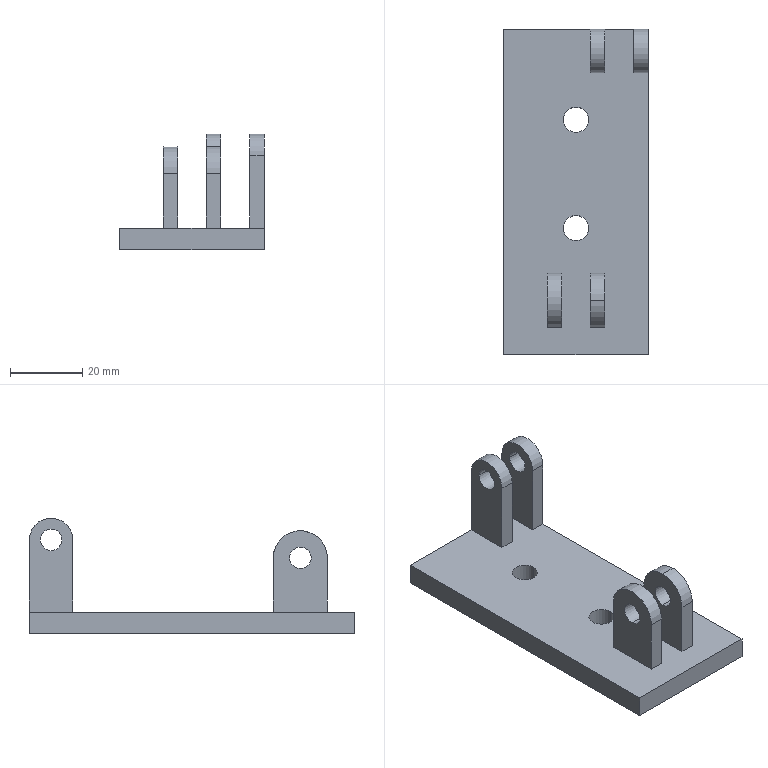Part | SolidWorks | features ICE 3, Extrusion 1, LPattern 1, MirrorPattern 1 | 1 solid | 36 faces | box 40 x 90 x 32 mm | volume 25565 mm3 | plane 19 | cylinder 17 | commonest cylinder face diameters 6 x8 7 x4 15 x3 12 x2
STEP:
#1=CARTESIAN_POINT('',(-3.5,20.,0.));
#2=VERTEX_POINT('',#1);
#3=CARTESIAN_POINT('',(3.5,20.,0.));
#4=VERTEX_POINT('',#3);
#5=CARTESIAN_POINT('',(0.,20.,0.));
#6=DIRECTION('',(0.,0.,1.));
#7=DIRECTION('',(1.,0.,0.));
#8=AXIS2_PLACEMENT_3D('',#5,#6,#7);
#9=CIRCLE('',#8,3.5);
#10=EDGE_CURVE('',#2,#4,#9,.T.);
#11=ORIENTED_EDGE('',*,*,#10,.F.);
#12=CARTESIAN_POINT('',(-3.5,20.,6.));
#13=VERTEX_POINT('',#12);
#14=CARTESIAN_POINT('',(-3.5,20.,0.));
#15=DIRECTION('',(0.,0.,1.));
#16=VECTOR('',#15,1000.);
#17=LINE('',#14,#16);
#18=EDGE_CURVE('',#2,#13,#17,.T.);
#19=ORIENTED_EDGE('',*,*,#18,.T.);
#20=CARTESIAN_POINT('',(3.5,20.,6.));
#21=VERTEX_POINT('',#20);
#22=CARTESIAN_POINT('',(0.,20.,6.));
#23=DIRECTION('',(0.,0.,1.));
#24=DIRECTION('',(1.,0.,0.));
#25=AXIS2_PLACEMENT_3D('',#22,#23,#24);
#26=CIRCLE('',#25,3.5);
#27=EDGE_CURVE('',#13,#21,#26,.T.);
#28=ORIENTED_EDGE('',*,*,#27,.T.);
#29=CARTESIAN_POINT('',(3.5,20.,0.));
#30=DIRECTION('',(0.,0.,1.));
#31=VECTOR('',#30,1000.);
#32=LINE('',#29,#31);
#33=EDGE_CURVE('',#4,#21,#32,.T.);
#34=ORIENTED_EDGE('',*,*,#33,.F.);
#35=EDGE_LOOP('',(#11,#19,#28,#34));
#36=FACE_OUTER_BOUND('',#35,.T.);
#37=CARTESIAN_POINT('',(0.,20.,0.));
#38=DIRECTION('',(0.,0.,1.));
#39=DIRECTION('',(1.,0.,0.));
#40=AXIS2_PLACEMENT_3D('',#37,#38,#39);
#41=CYLINDRICAL_SURFACE('',#40,3.5);
#42=ADVANCED_FACE('',(#36),#41,.F.);
#43=CARTESIAN_POINT('',(-3.5,-10.,0.));
#44=VERTEX_POINT('',#43);
#45=CARTESIAN_POINT('',(3.5,-10.,0.));
#46=VERTEX_POINT('',#45);
#47=CARTESIAN_POINT('',(0.,-10.,0.));
#48=DIRECTION('',(0.,0.,1.));
#49=DIRECTION('',(1.,0.,0.));
#50=AXIS2_PLACEMENT_3D('',#47,#48,#49);
#51=CIRCLE('',#50,3.5);
#52=EDGE_CURVE('',#44,#46,#51,.T.);
#53=ORIENTED_EDGE('',*,*,#52,.F.);
#54=CARTESIAN_POINT('',(-3.5,-10.,6.));
#55=VERTEX_POINT('',#54);
#56=CARTESIAN_POINT('',(-3.5,-10.,0.));
#57=DIRECTION('',(0.,0.,1.));
#58=VECTOR('',#57,1000.);
#59=LINE('',#56,#58);
#60=EDGE_CURVE('',#44,#55,#59,.T.);
#61=ORIENTED_EDGE('',*,*,#60,.T.);
#62=CARTESIAN_POINT('',(3.5,-10.,6.));
#63=VERTEX_POINT('',#62);
#64=CARTESIAN_POINT('',(0.,-10.,6.));
#65=DIRECTION('',(0.,0.,1.));
#66=DIRECTION('',(1.,0.,0.));
#67=AXIS2_PLACEMENT_3D('',#64,#65,#66);
#68=CIRCLE('',#67,3.5);
#69=EDGE_CURVE('',#55,#63,#68,.T.);
#70=ORIENTED_EDGE('',*,*,#69,.T.);
#71=CARTESIAN_POINT('',(3.5,-10.,0.));
#72=DIRECTION('',(0.,0.,1.));
#73=VECTOR('',#72,1000.);
#74=LINE('',#71,#73);
#75=EDGE_CURVE('',#46,#63,#74,.T.);
#76=ORIENTED_EDGE('',*,*,#75,.F.);
#77=EDGE_LOOP('',(#53,#61,#70,#76));
#78=FACE_OUTER_BOUND('',#77,.T.);
#79=CARTESIAN_POINT('',(0.,-10.,0.));
#80=DIRECTION('',(0.,0.,1.));
#81=DIRECTION('',(1.,0.,0.));
#82=AXIS2_PLACEMENT_3D('',#79,#80,#81);
#83=CYLINDRICAL_SURFACE('',#82,3.5);
#84=ADVANCED_FACE('',(#78),#83,.F.);
#85=CARTESIAN_POINT('',(4.,42.,26.));
#86=VERTEX_POINT('',#85);
#87=CARTESIAN_POINT('',(4.,36.,26.));
#88=VERTEX_POINT('',#87);
#89=CARTESIAN_POINT('',(4.,39.,26.));
#90=DIRECTION('',(-1.,0.,0.));
#91=DIRECTION('',(0.,-1.,0.));
#92=AXIS2_PLACEMENT_3D('',#89,#90,#91);
#93=CIRCLE('',#92,3.);
#94=EDGE_CURVE('',#86,#88,#93,.T.);
#95=ORIENTED_EDGE('',*,*,#94,.T.);
#96=CARTESIAN_POINT('',(8.,36.,26.));
#97=VERTEX_POINT('',#96);
#98=CARTESIAN_POINT('',(4.,36.,26.));
#99=DIRECTION('',(1.,0.,0.));
#100=VECTOR('',#99,1000.);
#101=LINE('',#98,#100);
#102=EDGE_CURVE('',#88,#97,#101,.T.);
#103=ORIENTED_EDGE('',*,*,#102,.T.);
#104=CARTESIAN_POINT('',(8.,42.,26.));
#105=VERTEX_POINT('',#104);
#106=CARTESIAN_POINT('',(8.,39.,26.));
#107=DIRECTION('',(-1.,0.,0.));
#108=DIRECTION('',(0.,-1.,0.));
#109=AXIS2_PLACEMENT_3D('',#106,#107,#108);
#110=CIRCLE('',#109,3.);
#111=EDGE_CURVE('',#105,#97,#110,.T.);
#112=ORIENTED_EDGE('',*,*,#111,.F.);
#113=CARTESIAN_POINT('',(4.,42.,26.));
#114=DIRECTION('',(1.,0.,0.));
#115=VECTOR('',#114,1000.);
#116=LINE('',#113,#115);
#117=EDGE_CURVE('',#86,#105,#116,.T.);
#118=ORIENTED_EDGE('',*,*,#117,.F.);
#119=EDGE_LOOP('',(#95,#103,#112,#118));
#120=FACE_OUTER_BOUND('',#119,.T.);
#121=CARTESIAN_POINT('',(4.,39.,26.));
#122=DIRECTION('',(1.,0.,0.));
#123=DIRECTION('',(0.,1.,0.));
#124=AXIS2_PLACEMENT_3D('',#121,#122,#123);
#125=CYLINDRICAL_SURFACE('',#124,3.);
#126=ADVANCED_FACE('',(#120),#125,.F.);
#127=CARTESIAN_POINT('',(-8.,-30.,24.));
#128=VERTEX_POINT('',#127);
#129=CARTESIAN_POINT('',(-8.,-30.,18.));
#130=VERTEX_POINT('',#129);
#131=CARTESIAN_POINT('',(-8.,-30.,21.));
#132=DIRECTION('',(1.,0.,0.));
#133=DIRECTION('',(0.,0.,-1.));
#134=AXIS2_PLACEMENT_3D('',#131,#132,#133);
#135=CIRCLE('',#134,3.);
#136=EDGE_CURVE('',#128,#130,#135,.T.);
#137=ORIENTED_EDGE('',*,*,#136,.F.);
#138=CARTESIAN_POINT('',(-4.,-30.,24.));
#139=VERTEX_POINT('',#138);
#140=CARTESIAN_POINT('',(-8.,-30.,24.));
#141=DIRECTION('',(1.,0.,0.));
#142=VECTOR('',#141,1000.);
#143=LINE('',#140,#142);
#144=EDGE_CURVE('',#128,#139,#143,.T.);
#145=ORIENTED_EDGE('',*,*,#144,.T.);
#146=CARTESIAN_POINT('',(-4.,-30.,18.));
#147=VERTEX_POINT('',#146);
#148=CARTESIAN_POINT('',(-4.,-30.,21.));
#149=DIRECTION('',(1.,0.,0.));
#150=DIRECTION('',(0.,0.,-1.));
#151=AXIS2_PLACEMENT_3D('',#148,#149,#150);
#152=CIRCLE('',#151,3.);
#153=EDGE_CURVE('',#139,#147,#152,.T.);
#154=ORIENTED_EDGE('',*,*,#153,.T.);
#155=CARTESIAN_POINT('',(-8.,-30.,18.));
#156=DIRECTION('',(1.,0.,0.));
#157=VECTOR('',#156,1000.);
#158=LINE('',#155,#157);
#159=EDGE_CURVE('',#130,#147,#158,.T.);
#160=ORIENTED_EDGE('',*,*,#159,.F.);
#161=EDGE_LOOP('',(#137,#145,#154,#160));
#162=FACE_OUTER_BOUND('',#161,.T.);
#163=CARTESIAN_POINT('',(-8.,-30.,21.));
#164=DIRECTION('',(1.,0.,0.));
#165=DIRECTION('',(0.,0.,-1.));
#166=AXIS2_PLACEMENT_3D('',#163,#164,#165);
#167=CYLINDRICAL_SURFACE('',#166,3.);
#168=ADVANCED_FACE('',(#162),#167,.F.);
#169=CARTESIAN_POINT('',(8.,-30.,24.));
#170=VERTEX_POINT('',#169);
#171=CARTESIAN_POINT('',(8.,-30.,18.));
#172=VERTEX_POINT('',#171);
#173=CARTESIAN_POINT('',(8.,-30.,21.));
#174=DIRECTION('',(1.,0.,0.));
#175=DIRECTION('',(0.,0.,-1.));
#176=AXIS2_PLACEMENT_3D('',#173,#174,#175);
#177=CIRCLE('',#176,3.);
#178=EDGE_CURVE('',#170,#172,#177,.T.);
#179=ORIENTED_EDGE('',*,*,#178,.T.);
#180=CARTESIAN_POINT('',(4.,-30.,18.));
#181=VERTEX_POINT('',#180);
#182=CARTESIAN_POINT('',(8.,-30.,18.));
#183=DIRECTION('',(-1.,0.,0.));
#184=VECTOR('',#183,1000.);
#185=LINE('',#182,#184);
#186=EDGE_CURVE('',#172,#181,#185,.T.);
#187=ORIENTED_EDGE('',*,*,#186,.T.);
#188=CARTESIAN_POINT('',(4.,-30.,24.));
#189=VERTEX_POINT('',#188);
#190=CARTESIAN_POINT('',(4.,-30.,21.));
#191=DIRECTION('',(1.,0.,0.));
#192=DIRECTION('',(0.,0.,-1.));
#193=AXIS2_PLACEMENT_3D('',#190,#191,#192);
#194=CIRCLE('',#193,3.);
#195=EDGE_CURVE('',#189,#181,#194,.T.);
#196=ORIENTED_EDGE('',*,*,#195,.F.);
#197=CARTESIAN_POINT('',(8.,-30.,24.));
#198=DIRECTION('',(-1.,0.,0.));
#199=VECTOR('',#198,1000.);
#200=LINE('',#197,#199);
#201=EDGE_CURVE('',#170,#189,#200,.T.);
#202=ORIENTED_EDGE('',*,*,#201,.F.);
#203=EDGE_LOOP('',(#179,#187,#196,#202));
#204=FACE_OUTER_BOUND('',#203,.T.);
#205=CARTESIAN_POINT('',(8.,-30.,21.));
#206=DIRECTION('',(-1.,0.,0.));
#207=DIRECTION('',(0.,0.,1.));
#208=AXIS2_PLACEMENT_3D('',#205,#206,#207);
#209=CYLINDRICAL_SURFACE('',#208,3.);
#210=ADVANCED_FACE('',(#204),#209,.F.);
#211=CARTESIAN_POINT('',(8.,-30.,28.5));
#212=VERTEX_POINT('',#211);
#213=CARTESIAN_POINT('',(8.,-37.5,21.));
#214=VERTEX_POINT('',#213);
#215=CARTESIAN_POINT('',(8.,-30.,21.));
#216=DIRECTION('',(1.,0.,0.));
#217=DIRECTION('',(0.,0.,-1.));
#218=AXIS2_PLACEMENT_3D('',#215,#216,#217);
#219=CIRCLE('',#218,7.5);
#220=EDGE_CURVE('',#212,#214,#219,.T.);
#221=ORIENTED_EDGE('',*,*,#220,.F.);
#222=CARTESIAN_POINT('',(4.,-30.,28.5));
#223=VERTEX_POINT('',#222);
#224=CARTESIAN_POINT('',(8.,-30.,28.5));
#225=DIRECTION('',(-1.,0.,0.));
#226=VECTOR('',#225,1000.);
#227=LINE('',#224,#226);
#228=EDGE_CURVE('',#212,#223,#227,.T.);
#229=ORIENTED_EDGE('',*,*,#228,.T.);
#230=CARTESIAN_POINT('',(4.,-37.5,21.));
#231=VERTEX_POINT('',#230);
#232=CARTESIAN_POINT('',(4.,-30.,21.));
#233=DIRECTION('',(1.,0.,0.));
#234=DIRECTION('',(0.,0.,-1.));
#235=AXIS2_PLACEMENT_3D('',#232,#233,#234);
#236=CIRCLE('',#235,7.5);
#237=EDGE_CURVE('',#223,#231,#236,.T.);
#238=ORIENTED_EDGE('',*,*,#237,.T.);
#239=CARTESIAN_POINT('',(8.,-37.5,21.));
#240=DIRECTION('',(-1.,0.,0.));
#241=VECTOR('',#240,1000.);
#242=LINE('',#239,#241);
#243=EDGE_CURVE('',#214,#231,#242,.T.);
#244=ORIENTED_EDGE('',*,*,#243,.F.);
#245=EDGE_LOOP('',(#221,#229,#238,#244));
#246=FACE_OUTER_BOUND('',#245,.T.);
#247=CARTESIAN_POINT('',(8.,-30.,21.));
#248=DIRECTION('',(-1.,0.,0.));
#249=DIRECTION('',(0.,0.,1.));
#250=AXIS2_PLACEMENT_3D('',#247,#248,#249);
#251=CYLINDRICAL_SURFACE('',#250,7.5);
#252=ADVANCED_FACE('',(#246),#251,.T.);
#253=CARTESIAN_POINT('',(16.,42.,26.));
#254=VERTEX_POINT('',#253);
#255=CARTESIAN_POINT('',(16.,36.,26.));
#256=VERTEX_POINT('',#255);
#257=CARTESIAN_POINT('',(16.,39.,26.));
#258=DIRECTION('',(-1.,0.,0.));
#259=DIRECTION('',(0.,-1.,0.));
#260=AXIS2_PLACEMENT_3D('',#257,#258,#259);
#261=CIRCLE('',#260,3.);
#262=EDGE_CURVE('',#254,#256,#261,.T.);
#263=ORIENTED_EDGE('',*,*,#262,.T.);
#264=CARTESIAN_POINT('',(20.,36.,26.));
#265=VERTEX_POINT('',#264);
#266=CARTESIAN_POINT('',(16.,36.,26.));
#267=DIRECTION('',(1.,0.,0.));
#268=VECTOR('',#267,1000.);
#269=LINE('',#266,#268);
#270=EDGE_CURVE('',#256,#265,#269,.T.);
#271=ORIENTED_EDGE('',*,*,#270,.T.);
#272=CARTESIAN_POINT('',(20.,42.,26.));
#273=VERTEX_POINT('',#272);
#274=CARTESIAN_POINT('',(20.,39.,26.));
#275=DIRECTION('',(-1.,0.,0.));
#276=DIRECTION('',(0.,-1.,0.));
#277=AXIS2_PLACEMENT_3D('',#274,#275,#276);
#278=CIRCLE('',#277,3.);
#279=EDGE_CURVE('',#273,#265,#278,.T.);
#280=ORIENTED_EDGE('',*,*,#279,.F.);
#281=CARTESIAN_POINT('',(16.,42.,26.));
#282=DIRECTION('',(1.,0.,0.));
#283=VECTOR('',#282,1000.);
#284=LINE('',#281,#283);
#285=EDGE_CURVE('',#254,#273,#284,.T.);
#286=ORIENTED_EDGE('',*,*,#285,.F.);
#287=EDGE_LOOP('',(#263,#271,#280,#286));
#288=FACE_OUTER_BOUND('',#287,.T.);
#289=CARTESIAN_POINT('',(16.,39.,26.));
#290=DIRECTION('',(1.,0.,0.));
#291=DIRECTION('',(0.,1.,0.));
#292=AXIS2_PLACEMENT_3D('',#289,#290,#291);
#293=CYLINDRICAL_SURFACE('',#292,3.);
#294=ADVANCED_FACE('',(#288),#293,.F.);
#295=CARTESIAN_POINT('',(0.,20.,6.));
#296=DIRECTION('',(0.,0.,1.));
#297=DIRECTION('',(1.,0.,0.));
#298=AXIS2_PLACEMENT_3D('',#295,#296,#297);
#299=CIRCLE('',#298,3.5);
#300=EDGE_CURVE('',#21,#13,#299,.T.);
#301=ORIENTED_EDGE('',*,*,#300,.F.);
#302=ORIENTED_EDGE('',*,*,#27,.F.);
#303=EDGE_LOOP('',(#301,#302));
#304=FACE_BOUND('',#303,.T.);
#305=CARTESIAN_POINT('',(0.,-10.,6.));
#306=DIRECTION('',(0.,0.,1.));
#307=DIRECTION('',(1.,0.,0.));
#308=AXIS2_PLACEMENT_3D('',#305,#306,#307);
#309=CIRCLE('',#308,3.5);
#310=EDGE_CURVE('',#63,#55,#309,.T.);
#311=ORIENTED_EDGE('',*,*,#310,.F.);
#312=ORIENTED_EDGE('',*,*,#69,.F.);
#313=EDGE_LOOP('',(#311,#312));
#314=FACE_BOUND('',#313,.T.);
#315=CARTESIAN_POINT('',(4.,45.,6.));
#316=VERTEX_POINT('',#315);
#317=CARTESIAN_POINT('',(4.,33.,6.));
#318=VERTEX_POINT('',#317);
#319=CARTESIAN_POINT('',(4.,45.,6.));
#320=DIRECTION('',(0.,-1.,0.));
#321=VECTOR('',#320,1000.);
#322=LINE('',#319,#321);
#323=EDGE_CURVE('',#316,#318,#322,.T.);
#324=ORIENTED_EDGE('',*,*,#323,.F.);
#325=CARTESIAN_POINT('',(-20.,45.,6.));
#326=VERTEX_POINT('',#325);
#327=CARTESIAN_POINT('',(-20.,45.,6.));
#328=DIRECTION('',(-1.,0.,0.));
#329=VECTOR('',#328,1000.);
#330=LINE('',#327,#329);
#331=EDGE_CURVE('',#316,#326,#330,.T.);
#332=ORIENTED_EDGE('',*,*,#331,.T.);
#333=CARTESIAN_POINT('',(-20.,-45.,6.));
#334=VERTEX_POINT('',#333);
#335=CARTESIAN_POINT('',(-20.,45.,6.));
#336=DIRECTION('',(0.,-1.,0.));
#337=VECTOR('',#336,1000.);
#338=LINE('',#335,#337);
#339=EDGE_CURVE('',#326,#334,#338,.T.);
#340=ORIENTED_EDGE('',*,*,#339,.T.);
#341=CARTESIAN_POINT('',(20.,-45.,6.));
#342=VERTEX_POINT('',#341);
#343=CARTESIAN_POINT('',(-20.,-45.,6.));
#344=DIRECTION('',(1.,0.,0.));
#345=VECTOR('',#344,1000.);
#346=LINE('',#343,#345);
#347=EDGE_CURVE('',#334,#342,#346,.T.);
#348=ORIENTED_EDGE('',*,*,#347,.T.);
#349=CARTESIAN_POINT('',(20.,33.,6.));
#350=VERTEX_POINT('',#349);
#351=CARTESIAN_POINT('',(20.,45.,6.));
#352=DIRECTION('',(0.,1.,0.));
#353=VECTOR('',#352,1000.);
#354=LINE('',#351,#353);
#355=EDGE_CURVE('',#342,#350,#354,.T.);
#356=ORIENTED_EDGE('',*,*,#355,.T.);
#357=CARTESIAN_POINT('',(16.,33.,6.));
#358=VERTEX_POINT('',#357);
#359=CARTESIAN_POINT('',(16.,33.,6.));
#360=DIRECTION('',(1.,0.,0.));
#361=VECTOR('',#360,1000.);
#362=LINE('',#359,#361);
#363=EDGE_CURVE('',#358,#350,#362,.T.);
#364=ORIENTED_EDGE('',*,*,#363,.F.);
#365=CARTESIAN_POINT('',(16.,45.,6.));
#366=VERTEX_POINT('',#365);
#367=CARTESIAN_POINT('',(16.,45.,6.));
#368=DIRECTION('',(0.,-1.,0.));
#369=VECTOR('',#368,1000.);
#370=LINE('',#367,#369);
#371=EDGE_CURVE('',#366,#358,#370,.T.);
#372=ORIENTED_EDGE('',*,*,#371,.F.);
#373=CARTESIAN_POINT('',(8.,45.,6.));
#374=VERTEX_POINT('',#373);
#375=CARTESIAN_POINT('',(-20.,45.,6.));
#376=DIRECTION('',(-1.,0.,0.));
#377=VECTOR('',#376,1000.);
#378=LINE('',#375,#377);
#379=EDGE_CURVE('',#366,#374,#378,.T.);
#380=ORIENTED_EDGE('',*,*,#379,.T.);
#381=CARTESIAN_POINT('',(8.,33.,6.));
#382=VERTEX_POINT('',#381);
#383=CARTESIAN_POINT('',(8.,45.,6.));
#384=DIRECTION('',(0.,-1.,0.));
#385=VECTOR('',#384,1000.);
#386=LINE('',#383,#385);
#387=EDGE_CURVE('',#374,#382,#386,.T.);
#388=ORIENTED_EDGE('',*,*,#387,.T.);
#389=CARTESIAN_POINT('',(4.,33.,6.));
#390=DIRECTION('',(1.,0.,0.));
#391=VECTOR('',#390,1000.);
#392=LINE('',#389,#391);
#393=EDGE_CURVE('',#318,#382,#392,.T.);
#394=ORIENTED_EDGE('',*,*,#393,.F.);
#395=EDGE_LOOP('',(#324,#332,#340,#348,#356,#364,#372,#380,#388,#394));
#396=FACE_OUTER_BOUND('',#395,.T.);
#397=CARTESIAN_POINT('',(-8.,-37.5,6.));
#398=VERTEX_POINT('',#397);
#399=CARTESIAN_POINT('',(-8.,-22.5,6.));
#400=VERTEX_POINT('',#399);
#401=CARTESIAN_POINT('',(-8.,-22.5,6.));
#402=DIRECTION('',(0.,1.,0.));
#403=VECTOR('',#402,1000.);
#404=LINE('',#401,#403);
#405=EDGE_CURVE('',#398,#400,#404,.T.);
#406=ORIENTED_EDGE('',*,*,#405,.T.);
#407=CARTESIAN_POINT('',(-4.,-22.5,6.));
#408=VERTEX_POINT('',#407);
#409=CARTESIAN_POINT('',(-8.,-22.5,6.));
#410=DIRECTION('',(1.,0.,0.));
#411=VECTOR('',#410,1000.);
#412=LINE('',#409,#411);
#413=EDGE_CURVE('',#400,#408,#412,.T.);
#414=ORIENTED_EDGE('',*,*,#413,.T.);
#415=CARTESIAN_POINT('',(-4.,-37.5,6.));
#416=VERTEX_POINT('',#415);
#417=CARTESIAN_POINT('',(-4.,-22.5,6.));
#418=DIRECTION('',(0.,1.,0.));
#419=VECTOR('',#418,1000.);
#420=LINE('',#417,#419);
#421=EDGE_CURVE('',#416,#408,#420,.T.);
#422=ORIENTED_EDGE('',*,*,#421,.F.);
#423=CARTESIAN_POINT('',(-8.,-37.5,6.));
#424=DIRECTION('',(1.,0.,0.));
#425=VECTOR('',#424,1000.);
#426=LINE('',#423,#425);
#427=EDGE_CURVE('',#398,#416,#426,.T.);
#428=ORIENTED_EDGE('',*,*,#427,.F.);
#429=EDGE_LOOP('',(#406,#414,#422,#428));
#430=FACE_BOUND('',#429,.T.);
#431=CARTESIAN_POINT('',(8.,-37.5,6.));
#432=VERTEX_POINT('',#431);
#433=CARTESIAN_POINT('',(8.,-22.5,6.));
#434=VERTEX_POINT('',#433);
#435=CARTESIAN_POINT('',(8.,-22.5,6.));
#436=DIRECTION('',(0.,1.,0.));
#437=VECTOR('',#436,1000.);
#438=LINE('',#435,#437);
#439=EDGE_CURVE('',#432,#434,#438,.T.);
#440=ORIENTED_EDGE('',*,*,#439,.F.);
#441=CARTESIAN_POINT('',(4.,-37.5,6.));
#442=VERTEX_POINT('',#441);
#443=CARTESIAN_POINT('',(8.,-37.5,6.));
#444=DIRECTION('',(-1.,0.,0.));
#445=VECTOR('',#444,1000.);
#446=LINE('',#443,#445);
#447=EDGE_CURVE('',#432,#442,#446,.T.);
#448=ORIENTED_EDGE('',*,*,#447,.T.);
#449=CARTESIAN_POINT('',(4.,-22.5,6.));
#450=VERTEX_POINT('',#449);
#451=CARTESIAN_POINT('',(4.,-22.5,6.));
#452=DIRECTION('',(0.,1.,0.));
#453=VECTOR('',#452,1000.);
#454=LINE('',#451,#453);
#455=EDGE_CURVE('',#442,#450,#454,.T.);
#456=ORIENTED_EDGE('',*,*,#455,.T.);
#457=CARTESIAN_POINT('',(8.,-22.5,6.));
#458=DIRECTION('',(-1.,0.,0.));
#459=VECTOR('',#458,1000.);
#460=LINE('',#457,#459);
#461=EDGE_CURVE('',#434,#450,#460,.T.);
#462=ORIENTED_EDGE('',*,*,#461,.F.);
#463=EDGE_LOOP('',(#440,#448,#456,#462));
#464=FACE_BOUND('',#463,.T.);
#465=CARTESIAN_POINT('',(0.,0.,6.));
#466=DIRECTION('',(0.,0.,1.));
#467=DIRECTION('',(1.,0.,0.));
#468=AXIS2_PLACEMENT_3D('',#465,#466,#467);
#469=PLANE('',#468);
#470=ADVANCED_FACE('',(#304,#314,#396,#430,#464),#469,.T.);
#471=CARTESIAN_POINT('',(20.,-45.,0.));
#472=VERTEX_POINT('',#471);
#473=CARTESIAN_POINT('',(20.,45.,0.));
#474=VERTEX_POINT('',#473);
#475=CARTESIAN_POINT('',(20.,45.,0.));
#476=DIRECTION('',(0.,1.,0.));
#477=VECTOR('',#476,1000.);
#478=LINE('',#475,#477);
#479=EDGE_CURVE('',#472,#474,#478,.T.);
#480=ORIENTED_EDGE('',*,*,#479,.T.);
#481=CARTESIAN_POINT('',(20.,45.,26.));
#482=VERTEX_POINT('',#481);
#483=CARTESIAN_POINT('',(20.,45.,6.));
#484=DIRECTION('',(0.,0.,-1.));
#485=VECTOR('',#484,1000.);
#486=LINE('',#483,#485);
#487=EDGE_CURVE('',#482,#474,#486,.T.);
#488=ORIENTED_EDGE('',*,*,#487,.F.);
#489=CARTESIAN_POINT('',(20.,33.,26.));
#490=VERTEX_POINT('',#489);
#491=CARTESIAN_POINT('',(20.,39.,26.));
#492=DIRECTION('',(-1.,0.,0.));
#493=DIRECTION('',(0.,-1.,0.));
#494=AXIS2_PLACEMENT_3D('',#491,#492,#493);
#495=CIRCLE('',#494,6.);
#496=EDGE_CURVE('',#490,#482,#495,.T.);
#497=ORIENTED_EDGE('',*,*,#496,.F.);
#498=CARTESIAN_POINT('',(20.,33.,6.));
#499=DIRECTION('',(0.,0.,1.));
#500=VECTOR('',#499,1000.);
#501=LINE('',#498,#500);
#502=EDGE_CURVE('',#350,#490,#501,.T.);
#503=ORIENTED_EDGE('',*,*,#502,.F.);
#504=ORIENTED_EDGE('',*,*,#355,.F.);
#505=CARTESIAN_POINT('',(20.,-45.,6.));
#506=DIRECTION('',(0.,0.,-1.));
#507=VECTOR('',#506,1000.);
#508=LINE('',#505,#507);
#509=EDGE_CURVE('',#342,#472,#508,.T.);
#510=ORIENTED_EDGE('',*,*,#509,.T.);
#511=EDGE_LOOP('',(#480,#488,#497,#503,#504,#510));
#512=FACE_OUTER_BOUND('',#511,.T.);
#513=ORIENTED_EDGE('',*,*,#279,.T.);
#514=CARTESIAN_POINT('',(20.,39.,26.));
#515=DIRECTION('',(-1.,0.,0.));
#516=DIRECTION('',(0.,-1.,0.));
#517=AXIS2_PLACEMENT_3D('',#514,#515,#516);
#518=CIRCLE('',#517,3.);
#519=EDGE_CURVE('',#265,#273,#518,.T.);
#520=ORIENTED_EDGE('',*,*,#519,.T.);
#521=EDGE_LOOP('',(#513,#520));
#522=FACE_BOUND('',#521,.T.);
#523=CARTESIAN_POINT('',(20.,45.,6.));
#524=DIRECTION('',(-1.,0.,0.));
#525=DIRECTION('',(0.,-1.,0.));
#526=AXIS2_PLACEMENT_3D('',#523,#524,#525);
#527=PLANE('',#526);
#528=ADVANCED_FACE('',(#512,#522),#527,.F.);
#529=CARTESIAN_POINT('',(-20.,45.,0.));
#530=VERTEX_POINT('',#529);
#531=CARTESIAN_POINT('',(-20.,45.,0.));
#532=DIRECTION('',(-1.,0.,0.));
#533=VECTOR('',#532,1000.);
#534=LINE('',#531,#533);
#535=EDGE_CURVE('',#474,#530,#534,.T.);
#536=ORIENTED_EDGE('',*,*,#535,.T.);
#537=CARTESIAN_POINT('',(-20.,45.,6.));
#538=DIRECTION('',(0.,0.,-1.));
#539=VECTOR('',#538,1000.);
#540=LINE('',#537,#539);
#541=EDGE_CURVE('',#326,#530,#540,.T.);
#542=ORIENTED_EDGE('',*,*,#541,.F.);
#543=ORIENTED_EDGE('',*,*,#331,.F.);
#544=CARTESIAN_POINT('',(4.,45.,26.));
#545=VERTEX_POINT('',#544);
#546=CARTESIAN_POINT('',(4.,45.,26.));
#547=DIRECTION('',(0.,0.,-1.));
#548=VECTOR('',#547,1000.);
#549=LINE('',#546,#548);
#550=EDGE_CURVE('',#545,#316,#549,.T.);
#551=ORIENTED_EDGE('',*,*,#550,.F.);
#552=CARTESIAN_POINT('',(8.,45.,26.));
#553=VERTEX_POINT('',#552);
#554=CARTESIAN_POINT('',(4.,45.,26.));
#555=DIRECTION('',(1.,0.,0.));
#556=VECTOR('',#555,1000.);
#557=LINE('',#554,#556);
#558=EDGE_CURVE('',#545,#553,#557,.T.);
#559=ORIENTED_EDGE('',*,*,#558,.T.);
#560=CARTESIAN_POINT('',(8.,45.,26.));
#561=DIRECTION('',(0.,0.,-1.));
#562=VECTOR('',#561,1000.);
#563=LINE('',#560,#562);
#564=EDGE_CURVE('',#553,#374,#563,.T.);
#565=ORIENTED_EDGE('',*,*,#564,.T.);
#566=ORIENTED_EDGE('',*,*,#379,.F.);
#567=CARTESIAN_POINT('',(16.,45.,26.));
#568=VERTEX_POINT('',#567);
#569=CARTESIAN_POINT('',(16.,45.,26.));
#570=DIRECTION('',(0.,0.,-1.));
#571=VECTOR('',#570,1000.);
#572=LINE('',#569,#571);
#573=EDGE_CURVE('',#568,#366,#572,.T.);
#574=ORIENTED_EDGE('',*,*,#573,.F.);
#575=CARTESIAN_POINT('',(16.,45.,26.));
#576=DIRECTION('',(1.,0.,0.));
#577=VECTOR('',#576,1000.);
#578=LINE('',#575,#577);
#579=EDGE_CURVE('',#568,#482,#578,.T.);
#580=ORIENTED_EDGE('',*,*,#579,.T.);
#581=ORIENTED_EDGE('',*,*,#487,.T.);
#582=EDGE_LOOP('',(#536,#542,#543,#551,#559,#565,#566,#574,#580,#581));
#583=FACE_OUTER_BOUND('',#582,.T.);
#584=CARTESIAN_POINT('',(-20.,45.,6.));
#585=DIRECTION('',(0.,-1.,0.));
#586=DIRECTION('',(0.,0.,-1.));
#587=AXIS2_PLACEMENT_3D('',#584,#585,#586);
#588=PLANE('',#587);
#589=ADVANCED_FACE('',(#583),#588,.F.);
#590=CARTESIAN_POINT('',(-20.,-45.,0.));
#591=VERTEX_POINT('',#590);
#592=CARTESIAN_POINT('',(-20.,45.,0.));
#593=DIRECTION('',(0.,-1.,0.));
#594=VECTOR('',#593,1000.);
#595=LINE('',#592,#594);
#596=EDGE_CURVE('',#530,#591,#595,.T.);
#597=ORIENTED_EDGE('',*,*,#596,.T.);
#598=CARTESIAN_POINT('',(-20.,-45.,6.));
#599=DIRECTION('',(0.,0.,-1.));
#600=VECTOR('',#599,1000.);
#601=LINE('',#598,#600);
#602=EDGE_CURVE('',#334,#591,#601,.T.);
#603=ORIENTED_EDGE('',*,*,#602,.F.);
#604=ORIENTED_EDGE('',*,*,#339,.F.);
#605=ORIENTED_EDGE('',*,*,#541,.T.);
#606=EDGE_LOOP('',(#597,#603,#604,#605));
#607=FACE_OUTER_BOUND('',#606,.T.);
#608=CARTESIAN_POINT('',(-20.,45.,6.));
#609=DIRECTION('',(1.,0.,0.));
#610=DIRECTION('',(0.,1.,0.));
#611=AXIS2_PLACEMENT_3D('',#608,#609,#610);
#612=PLANE('',#611);
#613=ADVANCED_FACE('',(#607),#612,.F.);
#614=CARTESIAN_POINT('',(-20.,-45.,0.));
#615=DIRECTION('',(1.,0.,0.));
#616=VECTOR('',#615,1000.);
#617=LINE('',#614,#616);
#618=EDGE_CURVE('',#591,#472,#617,.T.);
#619=ORIENTED_EDGE('',*,*,#618,.T.);
#620=ORIENTED_EDGE('',*,*,#509,.F.);
#621=ORIENTED_EDGE('',*,*,#347,.F.);
#622=ORIENTED_EDGE('',*,*,#602,.T.);
#623=EDGE_LOOP('',(#619,#620,#621,#622));
#624=FACE_OUTER_BOUND('',#623,.T.);
#625=CARTESIAN_POINT('',(-20.,-45.,6.));
#626=DIRECTION('',(0.,1.,0.));
#627=DIRECTION('',(0.,0.,1.));
#628=AXIS2_PLACEMENT_3D('',#625,#626,#627);
#629=PLANE('',#628);
#630=ADVANCED_FACE('',(#624),#629,.F.);
#631=CARTESIAN_POINT('',(0.,20.,0.));
#632=DIRECTION('',(0.,0.,1.));
#633=DIRECTION('',(1.,0.,0.));
#634=AXIS2_PLACEMENT_3D('',#631,#632,#633);
#635=CIRCLE('',#634,3.5);
#636=EDGE_CURVE('',#4,#2,#635,.T.);
#637=ORIENTED_EDGE('',*,*,#636,.T.);
#638=ORIENTED_EDGE('',*,*,#10,.T.);
#639=EDGE_LOOP('',(#637,#638));
#640=FACE_BOUND('',#639,.T.);
#641=CARTESIAN_POINT('',(0.,-10.,0.));
#642=DIRECTION('',(0.,0.,1.));
#643=DIRECTION('',(1.,0.,0.));
#644=AXIS2_PLACEMENT_3D('',#641,#642,#643);
#645=CIRCLE('',#644,3.5);
#646=EDGE_CURVE('',#46,#44,#645,.T.);
#647=ORIENTED_EDGE('',*,*,#646,.T.);
#648=ORIENTED_EDGE('',*,*,#52,.T.);
#649=EDGE_LOOP('',(#647,#648));
#650=FACE_BOUND('',#649,.T.);
#651=ORIENTED_EDGE('',*,*,#479,.F.);
#652=ORIENTED_EDGE('',*,*,#618,.F.);
#653=ORIENTED_EDGE('',*,*,#596,.F.);
#654=ORIENTED_EDGE('',*,*,#535,.F.);
#655=EDGE_LOOP('',(#651,#652,#653,#654));
#656=FACE_OUTER_BOUND('',#655,.T.);
#657=CARTESIAN_POINT('',(0.,0.,0.));
#658=DIRECTION('',(0.,0.,1.));
#659=DIRECTION('',(1.,0.,0.));
#660=AXIS2_PLACEMENT_3D('',#657,#658,#659);
#661=PLANE('',#660);
#662=ADVANCED_FACE('',(#640,#650,#656),#661,.F.);
#663=CARTESIAN_POINT('',(16.,33.,26.));
#664=VERTEX_POINT('',#663);
#665=CARTESIAN_POINT('',(16.,39.,26.));
#666=DIRECTION('',(-1.,0.,0.));
#667=DIRECTION('',(0.,-1.,0.));
#668=AXIS2_PLACEMENT_3D('',#665,#666,#667);
#669=CIRCLE('',#668,6.);
#670=EDGE_CURVE('',#664,#568,#669,.T.);
#671=ORIENTED_EDGE('',*,*,#670,.T.);
#672=ORIENTED_EDGE('',*,*,#573,.T.);
#673=ORIENTED_EDGE('',*,*,#371,.T.);
#674=CARTESIAN_POINT('',(16.,33.,6.));
#675=DIRECTION('',(0.,0.,1.));
#676=VECTOR('',#675,1000.);
#677=LINE('',#674,#676);
#678=EDGE_CURVE('',#358,#664,#677,.T.);
#679=ORIENTED_EDGE('',*,*,#678,.T.);
#680=EDGE_LOOP('',(#671,#672,#673,#679));
#681=FACE_OUTER_BOUND('',#680,.T.);
#682=ORIENTED_EDGE('',*,*,#262,.F.);
#683=CARTESIAN_POINT('',(16.,39.,26.));
#684=DIRECTION('',(-1.,0.,0.));
#685=DIRECTION('',(0.,-1.,0.));
#686=AXIS2_PLACEMENT_3D('',#683,#684,#685);
#687=CIRCLE('',#686,3.);
#688=EDGE_CURVE('',#256,#254,#687,.T.);
#689=ORIENTED_EDGE('',*,*,#688,.F.);
#690=EDGE_LOOP('',(#682,#689));
#691=FACE_BOUND('',#690,.T.);
#692=CARTESIAN_POINT('',(16.,39.,26.));
#693=DIRECTION('',(-1.,0.,0.));
#694=DIRECTION('',(0.,-1.,0.));
#695=AXIS2_PLACEMENT_3D('',#692,#693,#694);
#696=PLANE('',#695);
#697=ADVANCED_FACE('',(#681,#691),#696,.T.);
#698=ORIENTED_EDGE('',*,*,#496,.T.);
#699=ORIENTED_EDGE('',*,*,#579,.F.);
#700=ORIENTED_EDGE('',*,*,#670,.F.);
#701=CARTESIAN_POINT('',(16.,33.,26.));
#702=DIRECTION('',(1.,0.,0.));
#703=VECTOR('',#702,1000.);
#704=LINE('',#701,#703);
#705=EDGE_CURVE('',#664,#490,#704,.T.);
#706=ORIENTED_EDGE('',*,*,#705,.T.);
#707=EDGE_LOOP('',(#698,#699,#700,#706));
#708=FACE_OUTER_BOUND('',#707,.T.);
#709=CARTESIAN_POINT('',(16.,39.,26.));
#710=DIRECTION('',(1.,0.,0.));
#711=DIRECTION('',(0.,1.,0.));
#712=AXIS2_PLACEMENT_3D('',#709,#710,#711);
#713=CYLINDRICAL_SURFACE('',#712,6.);
#714=ADVANCED_FACE('',(#708),#713,.T.);
#715=ORIENTED_EDGE('',*,*,#502,.T.);
#716=ORIENTED_EDGE('',*,*,#705,.F.);
#717=ORIENTED_EDGE('',*,*,#678,.F.);
#718=ORIENTED_EDGE('',*,*,#363,.T.);
#719=EDGE_LOOP('',(#715,#716,#717,#718));
#720=FACE_OUTER_BOUND('',#719,.T.);
#721=CARTESIAN_POINT('',(16.,33.,6.));
#722=DIRECTION('',(0.,1.,0.));
#723=DIRECTION('',(-1.,0.,0.));
#724=AXIS2_PLACEMENT_3D('',#721,#722,#723);
#725=PLANE('',#724);
#726=ADVANCED_FACE('',(#720),#725,.F.);
#727=ORIENTED_EDGE('',*,*,#270,.F.);
#728=ORIENTED_EDGE('',*,*,#688,.T.);
#729=ORIENTED_EDGE('',*,*,#285,.T.);
#730=ORIENTED_EDGE('',*,*,#519,.F.);
#731=EDGE_LOOP('',(#727,#728,#729,#730));
#732=FACE_OUTER_BOUND('',#731,.T.);
#733=CARTESIAN_POINT('',(16.,39.,26.));
#734=DIRECTION('',(1.,0.,0.));
#735=DIRECTION('',(0.,1.,0.));
#736=AXIS2_PLACEMENT_3D('',#733,#734,#735);
#737=CYLINDRICAL_SURFACE('',#736,3.);
#738=ADVANCED_FACE('',(#732),#737,.F.);
#739=CARTESIAN_POINT('',(8.,-22.5,21.));
#740=VERTEX_POINT('',#739);
#741=CARTESIAN_POINT('',(8.,-30.,21.));
#742=DIRECTION('',(1.,0.,0.));
#743=DIRECTION('',(0.,0.,-1.));
#744=AXIS2_PLACEMENT_3D('',#741,#742,#743);
#745=CIRCLE('',#744,7.5);
#746=EDGE_CURVE('',#740,#212,#745,.T.);
#747=ORIENTED_EDGE('',*,*,#746,.T.);
#748=ORIENTED_EDGE('',*,*,#220,.T.);
#749=CARTESIAN_POINT('',(8.,-37.5,6.));
#750=DIRECTION('',(0.,0.,-1.));
#751=VECTOR('',#750,1000.);
#752=LINE('',#749,#751);
#753=EDGE_CURVE('',#214,#432,#752,.T.);
#754=ORIENTED_EDGE('',*,*,#753,.T.);
#755=ORIENTED_EDGE('',*,*,#439,.T.);
#756=CARTESIAN_POINT('',(8.,-22.5,21.));
#757=DIRECTION('',(0.,0.,1.));
#758=VECTOR('',#757,1000.);
#759=LINE('',#756,#758);
#760=EDGE_CURVE('',#434,#740,#759,.T.);
#761=ORIENTED_EDGE('',*,*,#760,.T.);
#762=EDGE_LOOP('',(#747,#748,#754,#755,#761));
#763=FACE_OUTER_BOUND('',#762,.T.);
#764=ORIENTED_EDGE('',*,*,#178,.F.);
#765=CARTESIAN_POINT('',(8.,-30.,21.));
#766=DIRECTION('',(1.,0.,0.));
#767=DIRECTION('',(0.,0.,-1.));
#768=AXIS2_PLACEMENT_3D('',#765,#766,#767);
#769=CIRCLE('',#768,3.);
#770=EDGE_CURVE('',#172,#170,#769,.T.);
#771=ORIENTED_EDGE('',*,*,#770,.F.);
#772=EDGE_LOOP('',(#764,#771));
#773=FACE_BOUND('',#772,.T.);
#774=CARTESIAN_POINT('',(8.,-30.,21.));
#775=DIRECTION('',(1.,0.,0.));
#776=DIRECTION('',(0.,0.,-1.));
#777=AXIS2_PLACEMENT_3D('',#774,#775,#776);
#778=PLANE('',#777);
#779=ADVANCED_FACE('',(#763,#773),#778,.T.);
#780=CARTESIAN_POINT('',(4.,-22.5,21.));
#781=VERTEX_POINT('',#780);
#782=CARTESIAN_POINT('',(4.,-30.,21.));
#783=DIRECTION('',(1.,0.,0.));
#784=DIRECTION('',(0.,0.,-1.));
#785=AXIS2_PLACEMENT_3D('',#782,#783,#784);
#786=CIRCLE('',#785,7.5);
#787=EDGE_CURVE('',#781,#223,#786,.T.);
#788=ORIENTED_EDGE('',*,*,#787,.F.);
#789=CARTESIAN_POINT('',(4.,-22.5,21.));
#790=DIRECTION('',(0.,0.,1.));
#791=VECTOR('',#790,1000.);
#792=LINE('',#789,#791);
#793=EDGE_CURVE('',#450,#781,#792,.T.);
#794=ORIENTED_EDGE('',*,*,#793,.F.);
#795=ORIENTED_EDGE('',*,*,#455,.F.);
#796=CARTESIAN_POINT('',(4.,-37.5,6.));
#797=DIRECTION('',(0.,0.,-1.));
#798=VECTOR('',#797,1000.);
#799=LINE('',#796,#798);
#800=EDGE_CURVE('',#231,#442,#799,.T.);
#801=ORIENTED_EDGE('',*,*,#800,.F.);
#802=ORIENTED_EDGE('',*,*,#237,.F.);
#803=EDGE_LOOP('',(#788,#794,#795,#801,#802));
#804=FACE_OUTER_BOUND('',#803,.T.);
#805=ORIENTED_EDGE('',*,*,#195,.T.);
#806=CARTESIAN_POINT('',(4.,-30.,21.));
#807=DIRECTION('',(1.,0.,0.));
#808=DIRECTION('',(0.,0.,-1.));
#809=AXIS2_PLACEMENT_3D('',#806,#807,#808);
#810=CIRCLE('',#809,3.);
#811=EDGE_CURVE('',#181,#189,#810,.T.);
#812=ORIENTED_EDGE('',*,*,#811,.T.);
#813=EDGE_LOOP('',(#805,#812));
#814=FACE_BOUND('',#813,.T.);
#815=CARTESIAN_POINT('',(4.,-30.,21.));
#816=DIRECTION('',(1.,0.,0.));
#817=DIRECTION('',(0.,0.,-1.));
#818=AXIS2_PLACEMENT_3D('',#815,#816,#817);
#819=PLANE('',#818);
#820=ADVANCED_FACE('',(#804,#814),#819,.F.);
#821=ORIENTED_EDGE('',*,*,#228,.F.);
#822=ORIENTED_EDGE('',*,*,#746,.F.);
#823=CARTESIAN_POINT('',(8.,-22.5,21.));
#824=DIRECTION('',(-1.,0.,0.));
#825=VECTOR('',#824,1000.);
#826=LINE('',#823,#825);
#827=EDGE_CURVE('',#740,#781,#826,.T.);
#828=ORIENTED_EDGE('',*,*,#827,.T.);
#829=ORIENTED_EDGE('',*,*,#787,.T.);
#830=EDGE_LOOP('',(#821,#822,#828,#829));
#831=FACE_OUTER_BOUND('',#830,.T.);
#832=CARTESIAN_POINT('',(8.,-30.,21.));
#833=DIRECTION('',(-1.,0.,0.));
#834=DIRECTION('',(0.,0.,1.));
#835=AXIS2_PLACEMENT_3D('',#832,#833,#834);
#836=CYLINDRICAL_SURFACE('',#835,7.5);
#837=ADVANCED_FACE('',(#831),#836,.T.);
#838=ORIENTED_EDGE('',*,*,#800,.T.);
#839=ORIENTED_EDGE('',*,*,#447,.F.);
#840=ORIENTED_EDGE('',*,*,#753,.F.);
#841=ORIENTED_EDGE('',*,*,#243,.T.);
#842=EDGE_LOOP('',(#838,#839,#840,#841));
#843=FACE_OUTER_BOUND('',#842,.T.);
#844=CARTESIAN_POINT('',(8.,-37.5,6.));
#845=DIRECTION('',(0.,1.,0.));
#846=DIRECTION('',(0.,0.,1.));
#847=AXIS2_PLACEMENT_3D('',#844,#845,#846);
#848=PLANE('',#847);
#849=ADVANCED_FACE('',(#843),#848,.F.);
#850=ORIENTED_EDGE('',*,*,#793,.T.);
#851=ORIENTED_EDGE('',*,*,#827,.F.);
#852=ORIENTED_EDGE('',*,*,#760,.F.);
#853=ORIENTED_EDGE('',*,*,#461,.T.);
#854=EDGE_LOOP('',(#850,#851,#852,#853));
#855=FACE_OUTER_BOUND('',#854,.T.);
#856=CARTESIAN_POINT('',(8.,-22.5,21.));
#857=DIRECTION('',(0.,-1.,0.));
#858=DIRECTION('',(0.,0.,-1.));
#859=AXIS2_PLACEMENT_3D('',#856,#857,#858);
#860=PLANE('',#859);
#861=ADVANCED_FACE('',(#855),#860,.F.);
#862=ORIENTED_EDGE('',*,*,#186,.F.);
#863=ORIENTED_EDGE('',*,*,#770,.T.);
#864=ORIENTED_EDGE('',*,*,#201,.T.);
#865=ORIENTED_EDGE('',*,*,#811,.F.);
#866=EDGE_LOOP('',(#862,#863,#864,#865));
#867=FACE_OUTER_BOUND('',#866,.T.);
#868=CARTESIAN_POINT('',(8.,-30.,21.));
#869=DIRECTION('',(-1.,0.,0.));
#870=DIRECTION('',(0.,0.,1.));
#871=AXIS2_PLACEMENT_3D('',#868,#869,#870);
#872=CYLINDRICAL_SURFACE('',#871,3.);
#873=ADVANCED_FACE('',(#867),#872,.F.);
#874=CARTESIAN_POINT('',(-4.,-22.5,21.));
#875=VERTEX_POINT('',#874);
#876=CARTESIAN_POINT('',(-4.,-37.5,21.));
#877=VERTEX_POINT('',#876);
#878=CARTESIAN_POINT('',(-4.,-30.,21.));
#879=DIRECTION('',(1.,0.,0.));
#880=DIRECTION('',(0.,0.,-1.));
#881=AXIS2_PLACEMENT_3D('',#878,#879,#880);
#882=CIRCLE('',#881,7.5);
#883=EDGE_CURVE('',#875,#877,#882,.T.);
#884=ORIENTED_EDGE('',*,*,#883,.F.);
#885=CARTESIAN_POINT('',(-8.,-22.5,21.));
#886=VERTEX_POINT('',#885);
#887=CARTESIAN_POINT('',(-8.,-22.5,21.));
#888=DIRECTION('',(1.,0.,0.));
#889=VECTOR('',#888,1000.);
#890=LINE('',#887,#889);
#891=EDGE_CURVE('',#886,#875,#890,.T.);
#892=ORIENTED_EDGE('',*,*,#891,.F.);
#893=CARTESIAN_POINT('',(-8.,-37.5,21.));
#894=VERTEX_POINT('',#893);
#895=CARTESIAN_POINT('',(-8.,-30.,21.));
#896=DIRECTION('',(1.,0.,0.));
#897=DIRECTION('',(0.,0.,-1.));
#898=AXIS2_PLACEMENT_3D('',#895,#896,#897);
#899=CIRCLE('',#898,7.5);
#900=EDGE_CURVE('',#886,#894,#899,.T.);
#901=ORIENTED_EDGE('',*,*,#900,.T.);
#902=CARTESIAN_POINT('',(-8.,-37.5,21.));
#903=DIRECTION('',(1.,0.,0.));
#904=VECTOR('',#903,1000.);
#905=LINE('',#902,#904);
#906=EDGE_CURVE('',#894,#877,#905,.T.);
#907=ORIENTED_EDGE('',*,*,#906,.T.);
#908=EDGE_LOOP('',(#884,#892,#901,#907));
#909=FACE_OUTER_BOUND('',#908,.T.);
#910=CARTESIAN_POINT('',(-8.,-30.,21.));
#911=DIRECTION('',(1.,0.,0.));
#912=DIRECTION('',(0.,0.,-1.));
#913=AXIS2_PLACEMENT_3D('',#910,#911,#912);
#914=CYLINDRICAL_SURFACE('',#913,7.5);
#915=ADVANCED_FACE('',(#909),#914,.T.);
#916=CARTESIAN_POINT('',(-4.,-22.5,21.));
#917=DIRECTION('',(0.,0.,1.));
#918=VECTOR('',#917,1000.);
#919=LINE('',#916,#918);
#920=EDGE_CURVE('',#408,#875,#919,.T.);
#921=ORIENTED_EDGE('',*,*,#920,.F.);
#922=ORIENTED_EDGE('',*,*,#413,.F.);
#923=CARTESIAN_POINT('',(-8.,-22.5,21.));
#924=DIRECTION('',(0.,0.,1.));
#925=VECTOR('',#924,1000.);
#926=LINE('',#923,#925);
#927=EDGE_CURVE('',#400,#886,#926,.T.);
#928=ORIENTED_EDGE('',*,*,#927,.T.);
#929=ORIENTED_EDGE('',*,*,#891,.T.);
#930=EDGE_LOOP('',(#921,#922,#928,#929));
#931=FACE_OUTER_BOUND('',#930,.T.);
#932=CARTESIAN_POINT('',(-8.,-22.5,21.));
#933=DIRECTION('',(0.,1.,0.));
#934=DIRECTION('',(0.,0.,1.));
#935=AXIS2_PLACEMENT_3D('',#932,#933,#934);
#936=PLANE('',#935);
#937=ADVANCED_FACE('',(#931),#936,.T.);
#938=CARTESIAN_POINT('',(-4.,-37.5,6.));
#939=DIRECTION('',(0.,0.,-1.));
#940=VECTOR('',#939,1000.);
#941=LINE('',#938,#940);
#942=EDGE_CURVE('',#877,#416,#941,.T.);
#943=ORIENTED_EDGE('',*,*,#942,.F.);
#944=ORIENTED_EDGE('',*,*,#906,.F.);
#945=CARTESIAN_POINT('',(-8.,-37.5,6.));
#946=DIRECTION('',(0.,0.,-1.));
#947=VECTOR('',#946,1000.);
#948=LINE('',#945,#947);
#949=EDGE_CURVE('',#894,#398,#948,.T.);
#950=ORIENTED_EDGE('',*,*,#949,.T.);
#951=ORIENTED_EDGE('',*,*,#427,.T.);
#952=EDGE_LOOP('',(#943,#944,#950,#951));
#953=FACE_OUTER_BOUND('',#952,.T.);
#954=CARTESIAN_POINT('',(-8.,-37.5,6.));
#955=DIRECTION('',(0.,-1.,0.));
#956=DIRECTION('',(0.,0.,-1.));
#957=AXIS2_PLACEMENT_3D('',#954,#955,#956);
#958=PLANE('',#957);
#959=ADVANCED_FACE('',(#953),#958,.T.);
#960=CARTESIAN_POINT('',(-8.,-30.,21.));
#961=DIRECTION('',(1.,0.,0.));
#962=DIRECTION('',(0.,0.,-1.));
#963=AXIS2_PLACEMENT_3D('',#960,#961,#962);
#964=CIRCLE('',#963,3.);
#965=EDGE_CURVE('',#130,#128,#964,.T.);
#966=ORIENTED_EDGE('',*,*,#965,.T.);
#967=ORIENTED_EDGE('',*,*,#136,.T.);
#968=EDGE_LOOP('',(#966,#967));
#969=FACE_BOUND('',#968,.T.);
#970=ORIENTED_EDGE('',*,*,#900,.F.);
#971=ORIENTED_EDGE('',*,*,#927,.F.);
#972=ORIENTED_EDGE('',*,*,#405,.F.);
#973=ORIENTED_EDGE('',*,*,#949,.F.);
#974=EDGE_LOOP('',(#970,#971,#972,#973));
#975=FACE_OUTER_BOUND('',#974,.T.);
#976=CARTESIAN_POINT('',(-8.,-30.,21.));
#977=DIRECTION('',(-1.,0.,0.));
#978=DIRECTION('',(0.,0.,-1.));
#979=AXIS2_PLACEMENT_3D('',#976,#977,#978);
#980=PLANE('',#979);
#981=ADVANCED_FACE('',(#969,#975),#980,.T.);
#982=CARTESIAN_POINT('',(-4.,-30.,21.));
#983=DIRECTION('',(1.,0.,0.));
#984=DIRECTION('',(0.,0.,-1.));
#985=AXIS2_PLACEMENT_3D('',#982,#983,#984);
#986=CIRCLE('',#985,3.);
#987=EDGE_CURVE('',#147,#139,#986,.T.);
#988=ORIENTED_EDGE('',*,*,#987,.F.);
#989=ORIENTED_EDGE('',*,*,#153,.F.);
#990=EDGE_LOOP('',(#988,#989));
#991=FACE_BOUND('',#990,.T.);
#992=ORIENTED_EDGE('',*,*,#883,.T.);
#993=ORIENTED_EDGE('',*,*,#942,.T.);
#994=ORIENTED_EDGE('',*,*,#421,.T.);
#995=ORIENTED_EDGE('',*,*,#920,.T.);
#996=EDGE_LOOP('',(#992,#993,#994,#995));
#997=FACE_OUTER_BOUND('',#996,.T.);
#998=CARTESIAN_POINT('',(-4.,-30.,21.));
#999=DIRECTION('',(-1.,0.,0.));
#1000=DIRECTION('',(0.,0.,-1.));
#1001=AXIS2_PLACEMENT_3D('',#998,#999,#1000);
#1002=PLANE('',#1001);
#1003=ADVANCED_FACE('',(#991,#997),#1002,.F.);
#1004=ORIENTED_EDGE('',*,*,#144,.F.);
#1005=ORIENTED_EDGE('',*,*,#965,.F.);
#1006=ORIENTED_EDGE('',*,*,#159,.T.);
#1007=ORIENTED_EDGE('',*,*,#987,.T.);
#1008=EDGE_LOOP('',(#1004,#1005,#1006,#1007));
#1009=FACE_OUTER_BOUND('',#1008,.T.);
#1010=CARTESIAN_POINT('',(-8.,-30.,21.));
#1011=DIRECTION('',(1.,0.,0.));
#1012=DIRECTION('',(0.,0.,-1.));
#1013=AXIS2_PLACEMENT_3D('',#1010,#1011,#1012);
#1014=CYLINDRICAL_SURFACE('',#1013,3.);
#1015=ADVANCED_FACE('',(#1009),#1014,.F.);
#1016=CARTESIAN_POINT('',(4.,33.,26.));
#1017=VERTEX_POINT('',#1016);
#1018=CARTESIAN_POINT('',(4.,39.,26.));
#1019=DIRECTION('',(-1.,0.,0.));
#1020=DIRECTION('',(0.,-1.,0.));
#1021=AXIS2_PLACEMENT_3D('',#1018,#1019,#1020);
#1022=CIRCLE('',#1021,6.);
#1023=EDGE_CURVE('',#1017,#545,#1022,.T.);
#1024=ORIENTED_EDGE('',*,*,#1023,.T.);
#1025=ORIENTED_EDGE('',*,*,#550,.T.);
#1026=ORIENTED_EDGE('',*,*,#323,.T.);
#1027=CARTESIAN_POINT('',(4.,33.,6.));
#1028=DIRECTION('',(0.,0.,1.));
#1029=VECTOR('',#1028,1000.);
#1030=LINE('',#1027,#1029);
#1031=EDGE_CURVE('',#318,#1017,#1030,.T.);
#1032=ORIENTED_EDGE('',*,*,#1031,.T.);
#1033=EDGE_LOOP('',(#1024,#1025,#1026,#1032));
#1034=FACE_OUTER_BOUND('',#1033,.T.);
#1035=ORIENTED_EDGE('',*,*,#94,.F.);
#1036=CARTESIAN_POINT('',(4.,39.,26.));
#1037=DIRECTION('',(-1.,0.,0.));
#1038=DIRECTION('',(0.,-1.,0.));
#1039=AXIS2_PLACEMENT_3D('',#1036,#1037,#1038);
#1040=CIRCLE('',#1039,3.);
#1041=EDGE_CURVE('',#88,#86,#1040,.T.);
#1042=ORIENTED_EDGE('',*,*,#1041,.F.);
#1043=EDGE_LOOP('',(#1035,#1042));
#1044=FACE_BOUND('',#1043,.T.);
#1045=CARTESIAN_POINT('',(4.,39.,26.));
#1046=DIRECTION('',(-1.,0.,0.));
#1047=DIRECTION('',(0.,-1.,0.));
#1048=AXIS2_PLACEMENT_3D('',#1045,#1046,#1047);
#1049=PLANE('',#1048);
#1050=ADVANCED_FACE('',(#1034,#1044),#1049,.T.);
#1051=CARTESIAN_POINT('',(8.,33.,26.));
#1052=VERTEX_POINT('',#1051);
#1053=CARTESIAN_POINT('',(8.,39.,26.));
#1054=DIRECTION('',(-1.,0.,0.));
#1055=DIRECTION('',(0.,-1.,0.));
#1056=AXIS2_PLACEMENT_3D('',#1053,#1054,#1055);
#1057=CIRCLE('',#1056,6.);
#1058=EDGE_CURVE('',#1052,#553,#1057,.T.);
#1059=ORIENTED_EDGE('',*,*,#1058,.F.);
#1060=CARTESIAN_POINT('',(8.,33.,6.));
#1061=DIRECTION('',(0.,0.,1.));
#1062=VECTOR('',#1061,1000.);
#1063=LINE('',#1060,#1062);
#1064=EDGE_CURVE('',#382,#1052,#1063,.T.);
#1065=ORIENTED_EDGE('',*,*,#1064,.F.);
#1066=ORIENTED_EDGE('',*,*,#387,.F.);
#1067=ORIENTED_EDGE('',*,*,#564,.F.);
#1068=EDGE_LOOP('',(#1059,#1065,#1066,#1067));
#1069=FACE_OUTER_BOUND('',#1068,.T.);
#1070=ORIENTED_EDGE('',*,*,#111,.T.);
#1071=CARTESIAN_POINT('',(8.,39.,26.));
#1072=DIRECTION('',(-1.,0.,0.));
#1073=DIRECTION('',(0.,-1.,0.));
#1074=AXIS2_PLACEMENT_3D('',#1071,#1072,#1073);
#1075=CIRCLE('',#1074,3.);
#1076=EDGE_CURVE('',#97,#105,#1075,.T.);
#1077=ORIENTED_EDGE('',*,*,#1076,.T.);
#1078=EDGE_LOOP('',(#1070,#1077));
#1079=FACE_BOUND('',#1078,.T.);
#1080=CARTESIAN_POINT('',(8.,39.,26.));
#1081=DIRECTION('',(-1.,0.,0.));
#1082=DIRECTION('',(0.,-1.,0.));
#1083=AXIS2_PLACEMENT_3D('',#1080,#1081,#1082);
#1084=PLANE('',#1083);
#1085=ADVANCED_FACE('',(#1069,#1079),#1084,.F.);
#1086=ORIENTED_EDGE('',*,*,#1058,.T.);
#1087=ORIENTED_EDGE('',*,*,#558,.F.);
#1088=ORIENTED_EDGE('',*,*,#1023,.F.);
#1089=CARTESIAN_POINT('',(4.,33.,26.));
#1090=DIRECTION('',(1.,0.,0.));
#1091=VECTOR('',#1090,1000.);
#1092=LINE('',#1089,#1091);
#1093=EDGE_CURVE('',#1017,#1052,#1092,.T.);
#1094=ORIENTED_EDGE('',*,*,#1093,.T.);
#1095=EDGE_LOOP('',(#1086,#1087,#1088,#1094));
#1096=FACE_OUTER_BOUND('',#1095,.T.);
#1097=CARTESIAN_POINT('',(4.,39.,26.));
#1098=DIRECTION('',(1.,0.,0.));
#1099=DIRECTION('',(0.,1.,0.));
#1100=AXIS2_PLACEMENT_3D('',#1097,#1098,#1099);
#1101=CYLINDRICAL_SURFACE('',#1100,6.);
#1102=ADVANCED_FACE('',(#1096),#1101,.T.);
#1103=ORIENTED_EDGE('',*,*,#1064,.T.);
#1104=ORIENTED_EDGE('',*,*,#1093,.F.);
#1105=ORIENTED_EDGE('',*,*,#1031,.F.);
#1106=ORIENTED_EDGE('',*,*,#393,.T.);
#1107=EDGE_LOOP('',(#1103,#1104,#1105,#1106));
#1108=FACE_OUTER_BOUND('',#1107,.T.);
#1109=CARTESIAN_POINT('',(4.,33.,6.));
#1110=DIRECTION('',(0.,1.,0.));
#1111=DIRECTION('',(-1.,0.,0.));
#1112=AXIS2_PLACEMENT_3D('',#1109,#1110,#1111);
#1113=PLANE('',#1112);
#1114=ADVANCED_FACE('',(#1108),#1113,.F.);
#1115=ORIENTED_EDGE('',*,*,#102,.F.);
#1116=ORIENTED_EDGE('',*,*,#1041,.T.);
#1117=ORIENTED_EDGE('',*,*,#117,.T.);
#1118=ORIENTED_EDGE('',*,*,#1076,.F.);
#1119=EDGE_LOOP('',(#1115,#1116,#1117,#1118));
#1120=FACE_OUTER_BOUND('',#1119,.T.);
#1121=CARTESIAN_POINT('',(4.,39.,26.));
#1122=DIRECTION('',(1.,0.,0.));
#1123=DIRECTION('',(0.,1.,0.));
#1124=AXIS2_PLACEMENT_3D('',#1121,#1122,#1123);
#1125=CYLINDRICAL_SURFACE('',#1124,3.);
#1126=ADVANCED_FACE('',(#1120),#1125,.F.);
#1127=ORIENTED_EDGE('',*,*,#60,.F.);
#1128=ORIENTED_EDGE('',*,*,#646,.F.);
#1129=ORIENTED_EDGE('',*,*,#75,.T.);
#1130=ORIENTED_EDGE('',*,*,#310,.T.);
#1131=EDGE_LOOP('',(#1127,#1128,#1129,#1130));
#1132=FACE_OUTER_BOUND('',#1131,.T.);
#1133=CARTESIAN_POINT('',(0.,-10.,0.));
#1134=DIRECTION('',(0.,0.,1.));
#1135=DIRECTION('',(1.,0.,0.));
#1136=AXIS2_PLACEMENT_3D('',#1133,#1134,#1135);
#1137=CYLINDRICAL_SURFACE('',#1136,3.5);
#1138=ADVANCED_FACE('',(#1132),#1137,.F.);
#1139=ORIENTED_EDGE('',*,*,#18,.F.);
#1140=ORIENTED_EDGE('',*,*,#636,.F.);
#1141=ORIENTED_EDGE('',*,*,#33,.T.);
#1142=ORIENTED_EDGE('',*,*,#300,.T.);
#1143=EDGE_LOOP('',(#1139,#1140,#1141,#1142));
#1144=FACE_OUTER_BOUND('',#1143,.T.);
#1145=CARTESIAN_POINT('',(0.,20.,0.));
#1146=DIRECTION('',(0.,0.,1.));
#1147=DIRECTION('',(1.,0.,0.));
#1148=AXIS2_PLACEMENT_3D('',#1145,#1146,#1147);
#1149=CYLINDRICAL_SURFACE('',#1148,3.5);
#1150=ADVANCED_FACE('',(#1144),#1149,.F.);
#1151=CLOSED_SHELL('',(#42,#84,#126,#168,#210,#252,#294,#470,#528,#589,#613,#630,#662,#697,#714,#726,#738,#779,#820,#837,#849,#861,#873,#915,#937,#959,#981,#1003,#1015,#1050,#1085,#1102,#1114,#1126,#1138,#1150));
#1152=MANIFOLD_SOLID_BREP('',#1151);
#1153=CARTESIAN_POINT('',(0.,0.,0.));
#1154=DIRECTION('',(0.,0.,1.));
#1155=DIRECTION('',(1.,0.,0.));
#1156=AXIS2_PLACEMENT_3D('',#1153,#1154,#1155);
#1157=(LENGTH_UNIT()NAMED_UNIT(*)SI_UNIT(.MILLI.,.METRE.));
#1158=UNCERTAINTY_MEASURE_WITH_UNIT(LENGTH_MEASURE(0.00001),#1157,'','');
#1159=(NAMED_UNIT(*)PLANE_ANGLE_UNIT()SI_UNIT($,.RADIAN.));
#1160=(NAMED_UNIT(*)SI_UNIT($,.STERADIAN.)SOLID_ANGLE_UNIT());
#1161=(GEOMETRIC_REPRESENTATION_CONTEXT(3)GLOBAL_UNCERTAINTY_ASSIGNED_CONTEXT((#1158))GLOBAL_UNIT_ASSIGNED_CONTEXT((#1157,#1159,#1160))REPRESENTATION_CONTEXT('',''));
#1162=ADVANCED_BREP_SHAPE_REPRESENTATION('',(#1152,#1156),#1161);